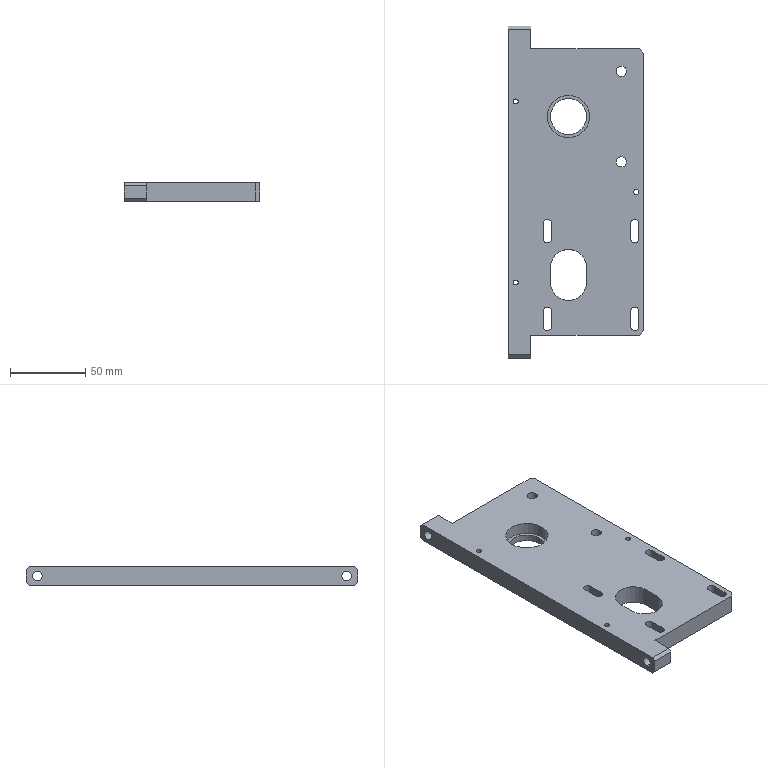Part | SolidWorks | features ICE 7, HoleWzd 3, Chamfer 2, Extrusion 1 | 1 solid | 75 faces | box 90 x 220 x 12.5 mm | volume 194769 mm3 | plane 39 | cylinder 36 | commonest cylinder face diameters 5.5 x8 10 x8 3.3 x6 6.5 x4 6.8 x4 24 x4